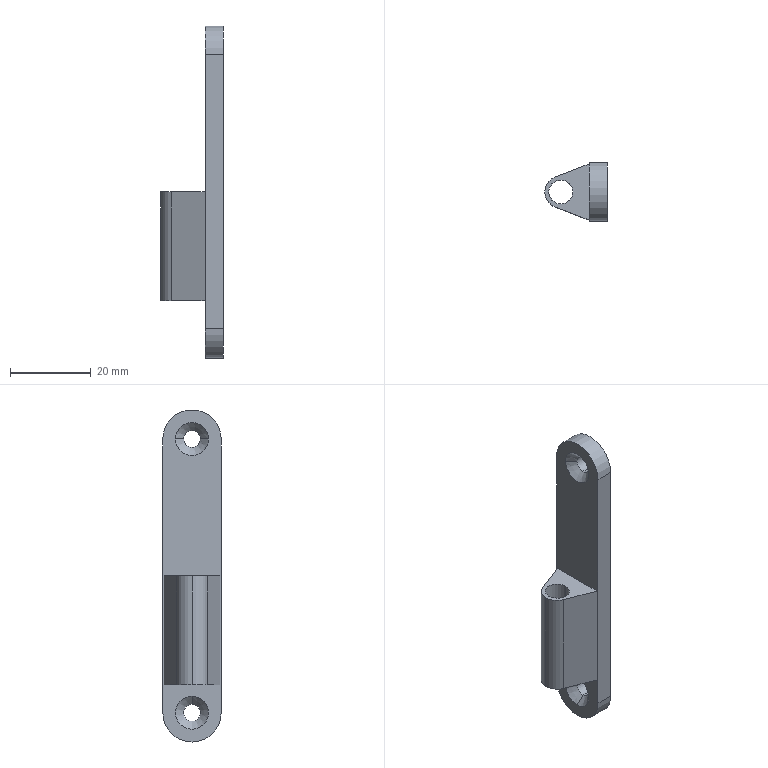Part | SolidWorks | features BaseBody 1 | 1 solid | 23 faces | box 15.5 x 14.5 x 82.5 mm | volume 7031 mm3 | cylinder 11 | plane 8 | cone 4 | commonest cylinder face diameters 4.2 x4 14.5 x3 6 x2 8 x2
STEP:
#1=CARTESIAN_POINT('',(11.5,0.,-36.1));
#2=VERTEX_POINT('',#1);
#3=CARTESIAN_POINT('',(11.5,0.,-31.9));
#4=VERTEX_POINT('',#3);
#5=CARTESIAN_POINT('',(11.5,0.,-34.));
#6=DIRECTION('',(-1.,0.,0.));
#7=DIRECTION('',(0.,0.,1.));
#8=AXIS2_PLACEMENT_3D('',#5,#6,#7);
#9=CIRCLE('',#8,2.1);
#10=EDGE_CURVE('',#2,#4,#9,.T.);
#11=ORIENTED_EDGE('',*,*,#10,.F.);
#12=CARTESIAN_POINT('',(9.,0.,-36.1));
#13=VERTEX_POINT('',#12);
#14=CARTESIAN_POINT('',(11.5,0.,-36.1));
#15=DIRECTION('',(-1.,0.,0.));
#16=VECTOR('',#15,1000.);
#17=LINE('',#14,#16);
#18=EDGE_CURVE('',#2,#13,#17,.T.);
#19=ORIENTED_EDGE('',*,*,#18,.T.);
#20=CARTESIAN_POINT('',(9.,0.,-31.9));
#21=VERTEX_POINT('',#20);
#22=CARTESIAN_POINT('',(9.,0.,-34.));
#23=DIRECTION('',(1.,0.,0.));
#24=DIRECTION('',(0.,0.,1.));
#25=AXIS2_PLACEMENT_3D('',#22,#23,#24);
#26=CIRCLE('',#25,2.1);
#27=EDGE_CURVE('',#21,#13,#26,.T.);
#28=ORIENTED_EDGE('',*,*,#27,.F.);
#29=CARTESIAN_POINT('',(11.5,0.,-31.9));
#30=DIRECTION('',(-1.,0.,0.));
#31=VECTOR('',#30,1000.);
#32=LINE('',#29,#31);
#33=EDGE_CURVE('',#4,#21,#32,.T.);
#34=ORIENTED_EDGE('',*,*,#33,.F.);
#35=EDGE_LOOP('',(#11,#19,#28,#34));
#36=FACE_OUTER_BOUND('',#35,.T.);
#37=CARTESIAN_POINT('',(11.5,0.,-34.));
#38=DIRECTION('',(-1.,0.,0.));
#39=DIRECTION('',(0.,0.,1.));
#40=AXIS2_PLACEMENT_3D('',#37,#38,#39);
#41=CYLINDRICAL_SURFACE('',#40,2.1);
#42=ADVANCED_FACE('',(#36),#41,.F.);
#43=CARTESIAN_POINT('',(7.,-7.25,-34.));
#44=VERTEX_POINT('',#43);
#45=CARTESIAN_POINT('',(7.,0.,-41.25));
#46=VERTEX_POINT('',#45);
#47=CARTESIAN_POINT('',(7.,0.,-34.));
#48=DIRECTION('',(1.,0.,0.));
#49=DIRECTION('',(0.,0.,-1.));
#50=AXIS2_PLACEMENT_3D('',#47,#48,#49);
#51=CIRCLE('',#50,7.25);
#52=EDGE_CURVE('',#44,#46,#51,.T.);
#53=ORIENTED_EDGE('',*,*,#52,.T.);
#54=CARTESIAN_POINT('',(11.5,0.,-41.25));
#55=VERTEX_POINT('',#54);
#56=CARTESIAN_POINT('',(11.5,0.,-41.25));
#57=DIRECTION('',(1.,0.,0.));
#58=VECTOR('',#57,1000.);
#59=LINE('',#56,#58);
#60=EDGE_CURVE('',#46,#55,#59,.T.);
#61=ORIENTED_EDGE('',*,*,#60,.T.);
#62=CARTESIAN_POINT('',(11.5,-7.25,-34.));
#63=VERTEX_POINT('',#62);
#64=CARTESIAN_POINT('',(11.5,0.,-34.));
#65=DIRECTION('',(1.,0.,0.));
#66=DIRECTION('',(0.,0.,-1.));
#67=AXIS2_PLACEMENT_3D('',#64,#65,#66);
#68=CIRCLE('',#67,7.25);
#69=EDGE_CURVE('',#63,#55,#68,.T.);
#70=ORIENTED_EDGE('',*,*,#69,.F.);
#71=CARTESIAN_POINT('',(11.5,-7.25,-34.));
#72=DIRECTION('',(-1.,0.,0.));
#73=VECTOR('',#72,1000.);
#74=LINE('',#71,#73);
#75=EDGE_CURVE('',#63,#44,#74,.T.);
#76=ORIENTED_EDGE('',*,*,#75,.T.);
#77=EDGE_LOOP('',(#53,#61,#70,#76));
#78=FACE_OUTER_BOUND('',#77,.T.);
#79=CARTESIAN_POINT('',(11.5,0.,-34.));
#80=DIRECTION('',(1.,0.,0.));
#81=DIRECTION('',(0.,0.,-1.));
#82=AXIS2_PLACEMENT_3D('',#79,#80,#81);
#83=CYLINDRICAL_SURFACE('',#82,7.25);
#84=ADVANCED_FACE('',(#78),#83,.T.);
#85=CARTESIAN_POINT('',(11.5,0.,31.9));
#86=VERTEX_POINT('',#85);
#87=CARTESIAN_POINT('',(11.5,0.,36.1));
#88=VERTEX_POINT('',#87);
#89=CARTESIAN_POINT('',(11.5,0.,34.));
#90=DIRECTION('',(-1.,0.,0.));
#91=DIRECTION('',(0.,0.,1.));
#92=AXIS2_PLACEMENT_3D('',#89,#90,#91);
#93=CIRCLE('',#92,2.1);
#94=EDGE_CURVE('',#86,#88,#93,.T.);
#95=ORIENTED_EDGE('',*,*,#94,.F.);
#96=CARTESIAN_POINT('',(9.,0.,31.9));
#97=VERTEX_POINT('',#96);
#98=CARTESIAN_POINT('',(11.5,0.,31.9));
#99=DIRECTION('',(-1.,0.,0.));
#100=VECTOR('',#99,1000.);
#101=LINE('',#98,#100);
#102=EDGE_CURVE('',#86,#97,#101,.T.);
#103=ORIENTED_EDGE('',*,*,#102,.T.);
#104=CARTESIAN_POINT('',(9.,-2.1,34.));
#105=VERTEX_POINT('',#104);
#106=CARTESIAN_POINT('',(9.,0.,34.));
#107=DIRECTION('',(1.,0.,0.));
#108=DIRECTION('',(0.,0.,1.));
#109=AXIS2_PLACEMENT_3D('',#106,#107,#108);
#110=CIRCLE('',#109,2.1);
#111=EDGE_CURVE('',#105,#97,#110,.T.);
#112=ORIENTED_EDGE('',*,*,#111,.F.);
#113=CARTESIAN_POINT('',(9.,0.,36.1));
#114=VERTEX_POINT('',#113);
#115=CARTESIAN_POINT('',(9.,0.,34.));
#116=DIRECTION('',(1.,0.,0.));
#117=DIRECTION('',(0.,0.,1.));
#118=AXIS2_PLACEMENT_3D('',#115,#116,#117);
#119=CIRCLE('',#118,2.1);
#120=EDGE_CURVE('',#114,#105,#119,.T.);
#121=ORIENTED_EDGE('',*,*,#120,.F.);
#122=CARTESIAN_POINT('',(11.5,0.,36.1));
#123=DIRECTION('',(-1.,0.,0.));
#124=VECTOR('',#123,1000.);
#125=LINE('',#122,#124);
#126=EDGE_CURVE('',#88,#114,#125,.T.);
#127=ORIENTED_EDGE('',*,*,#126,.F.);
#128=EDGE_LOOP('',(#95,#103,#112,#121,#127));
#129=FACE_OUTER_BOUND('',#128,.T.);
#130=CARTESIAN_POINT('',(11.5,0.,34.));
#131=DIRECTION('',(-1.,0.,0.));
#132=DIRECTION('',(0.,0.,1.));
#133=AXIS2_PLACEMENT_3D('',#130,#131,#132);
#134=CYLINDRICAL_SURFACE('',#133,2.1);
#135=ADVANCED_FACE('',(#129),#134,.F.);
#136=ORIENTED_EDGE('',*,*,#27,.T.);
#137=CARTESIAN_POINT('',(7.,0.,-38.1));
#138=VERTEX_POINT('',#137);
#139=CARTESIAN_POINT('',(7.,0.,-38.1));
#140=DIRECTION('',(-0.7071,0.,-0.7071));
#141=VECTOR('',#140,1000.);
#142=LINE('',#139,#141);
#143=EDGE_CURVE('',#13,#138,#142,.T.);
#144=ORIENTED_EDGE('',*,*,#143,.T.);
#145=CARTESIAN_POINT('',(7.,0.,-29.9));
#146=VERTEX_POINT('',#145);
#147=CARTESIAN_POINT('',(7.,0.,-34.));
#148=DIRECTION('',(1.,0.,0.));
#149=DIRECTION('',(0.,0.,1.));
#150=AXIS2_PLACEMENT_3D('',#147,#148,#149);
#151=CIRCLE('',#150,4.1);
#152=EDGE_CURVE('',#146,#138,#151,.T.);
#153=ORIENTED_EDGE('',*,*,#152,.F.);
#154=CARTESIAN_POINT('',(7.,0.,-29.9));
#155=DIRECTION('',(-0.7071,0.,0.7071));
#156=VECTOR('',#155,1000.);
#157=LINE('',#154,#156);
#158=EDGE_CURVE('',#21,#146,#157,.T.);
#159=ORIENTED_EDGE('',*,*,#158,.F.);
#160=EDGE_LOOP('',(#136,#144,#153,#159));
#161=FACE_OUTER_BOUND('',#160,.T.);
#162=CARTESIAN_POINT('',(7.,0.,-34.));
#163=DIRECTION('',(-1.,0.,0.));
#164=DIRECTION('',(0.,0.,1.));
#165=AXIS2_PLACEMENT_3D('',#162,#163,#164);
#166=CONICAL_SURFACE('',#165,4.1,0.7854);
#167=ADVANCED_FACE('',(#161),#166,.F.);
#168=ORIENTED_EDGE('',*,*,#111,.T.);
#169=CARTESIAN_POINT('',(9.,2.1,34.));
#170=VERTEX_POINT('',#169);
#171=CARTESIAN_POINT('',(9.,0.,34.));
#172=DIRECTION('',(1.,0.,0.));
#173=DIRECTION('',(0.,0.,1.));
#174=AXIS2_PLACEMENT_3D('',#171,#172,#173);
#175=CIRCLE('',#174,2.1);
#176=EDGE_CURVE('',#97,#170,#175,.T.);
#177=ORIENTED_EDGE('',*,*,#176,.T.);
#178=CARTESIAN_POINT('',(7.,4.1,34.));
#179=VERTEX_POINT('',#178);
#180=CARTESIAN_POINT('',(7.,4.1,34.));
#181=DIRECTION('',(-0.7071,0.7071,0.));
#182=VECTOR('',#181,1000.);
#183=LINE('',#180,#182);
#184=EDGE_CURVE('',#170,#179,#183,.T.);
#185=ORIENTED_EDGE('',*,*,#184,.T.);
#186=CARTESIAN_POINT('',(7.,-4.1,34.));
#187=VERTEX_POINT('',#186);
#188=CARTESIAN_POINT('',(7.,0.,34.));
#189=DIRECTION('',(-1.,0.,0.));
#190=DIRECTION('',(0.,-1.,0.));
#191=AXIS2_PLACEMENT_3D('',#188,#189,#190);
#192=CIRCLE('',#191,4.1);
#193=EDGE_CURVE('',#179,#187,#192,.T.);
#194=ORIENTED_EDGE('',*,*,#193,.T.);
#195=CARTESIAN_POINT('',(7.,-4.1,34.));
#196=DIRECTION('',(-0.7071,-0.7071,0.));
#197=VECTOR('',#196,1000.);
#198=LINE('',#195,#197);
#199=EDGE_CURVE('',#105,#187,#198,.T.);
#200=ORIENTED_EDGE('',*,*,#199,.F.);
#201=EDGE_LOOP('',(#168,#177,#185,#194,#200));
#202=FACE_OUTER_BOUND('',#201,.T.);
#203=CARTESIAN_POINT('',(7.,0.,34.));
#204=DIRECTION('',(-1.,0.,0.));
#205=DIRECTION('',(0.,-1.,0.));
#206=AXIS2_PLACEMENT_3D('',#203,#204,#205);
#207=CONICAL_SURFACE('',#206,4.1,0.7854);
#208=ADVANCED_FACE('',(#202),#207,.F.);
#209=CARTESIAN_POINT('',(-4.,0.,0.));
#210=VERTEX_POINT('',#209);
#211=CARTESIAN_POINT('',(-1.425,-3.738,0.));
#212=VERTEX_POINT('',#211);
#213=CARTESIAN_POINT('',(0.,0.,0.));
#214=DIRECTION('',(0.,0.,1.));
#215=DIRECTION('',(-1.,0.,0.));
#216=AXIS2_PLACEMENT_3D('',#213,#214,#215);
#217=CIRCLE('',#216,4.);
#218=EDGE_CURVE('',#210,#212,#217,.T.);
#219=ORIENTED_EDGE('',*,*,#218,.F.);
#220=CARTESIAN_POINT('',(-4.,0.,-27.));
#221=VERTEX_POINT('',#220);
#222=CARTESIAN_POINT('',(-4.,0.,-27.));
#223=DIRECTION('',(0.,0.,-1.));
#224=VECTOR('',#223,1000.);
#225=LINE('',#222,#224);
#226=EDGE_CURVE('',#210,#221,#225,.T.);
#227=ORIENTED_EDGE('',*,*,#226,.T.);
#228=CARTESIAN_POINT('',(-1.425,-3.738,-27.));
#229=VERTEX_POINT('',#228);
#230=CARTESIAN_POINT('',(0.,0.,-27.));
#231=DIRECTION('',(0.,0.,1.));
#232=DIRECTION('',(-1.,0.,0.));
#233=AXIS2_PLACEMENT_3D('',#230,#231,#232);
#234=CIRCLE('',#233,4.);
#235=EDGE_CURVE('',#221,#229,#234,.T.);
#236=ORIENTED_EDGE('',*,*,#235,.T.);
#237=CARTESIAN_POINT('',(-1.425,-3.738,-27.));
#238=DIRECTION('',(0.,0.,-1.));
#239=VECTOR('',#238,1000.);
#240=LINE('',#237,#239);
#241=EDGE_CURVE('',#212,#229,#240,.T.);
#242=ORIENTED_EDGE('',*,*,#241,.F.);
#243=EDGE_LOOP('',(#219,#227,#236,#242));
#244=FACE_OUTER_BOUND('',#243,.T.);
#245=CARTESIAN_POINT('',(0.,0.,-27.));
#246=DIRECTION('',(0.,0.,-1.));
#247=DIRECTION('',(-1.,0.,0.));
#248=AXIS2_PLACEMENT_3D('',#245,#246,#247);
#249=CYLINDRICAL_SURFACE('',#248,4.);
#250=ADVANCED_FACE('',(#244),#249,.T.);
#251=CARTESIAN_POINT('',(3.,0.,0.));
#252=VERTEX_POINT('',#251);
#253=CARTESIAN_POINT('',(-3.,0.,0.));
#254=VERTEX_POINT('',#253);
#255=CARTESIAN_POINT('',(0.,0.,0.));
#256=DIRECTION('',(0.,0.,-1.));
#257=DIRECTION('',(-1.,0.,0.));
#258=AXIS2_PLACEMENT_3D('',#255,#256,#257);
#259=CIRCLE('',#258,3.);
#260=EDGE_CURVE('',#252,#254,#259,.T.);
#261=ORIENTED_EDGE('',*,*,#260,.F.);
#262=CARTESIAN_POINT('',(3.,0.,-27.));
#263=VERTEX_POINT('',#262);
#264=CARTESIAN_POINT('',(3.,0.,-27.));
#265=DIRECTION('',(0.,0.,-1.));
#266=VECTOR('',#265,1000.);
#267=LINE('',#264,#266);
#268=EDGE_CURVE('',#252,#263,#267,.T.);
#269=ORIENTED_EDGE('',*,*,#268,.T.);
#270=CARTESIAN_POINT('',(-3.,0.,-27.));
#271=VERTEX_POINT('',#270);
#272=CARTESIAN_POINT('',(0.,0.,-27.));
#273=DIRECTION('',(0.,0.,-1.));
#274=DIRECTION('',(-1.,0.,0.));
#275=AXIS2_PLACEMENT_3D('',#272,#273,#274);
#276=CIRCLE('',#275,3.);
#277=EDGE_CURVE('',#263,#271,#276,.T.);
#278=ORIENTED_EDGE('',*,*,#277,.T.);
#279=CARTESIAN_POINT('',(-3.,0.,-27.));
#280=DIRECTION('',(0.,0.,-1.));
#281=VECTOR('',#280,1000.);
#282=LINE('',#279,#281);
#283=EDGE_CURVE('',#254,#271,#282,.T.);
#284=ORIENTED_EDGE('',*,*,#283,.F.);
#285=EDGE_LOOP('',(#261,#269,#278,#284));
#286=FACE_OUTER_BOUND('',#285,.T.);
#287=CARTESIAN_POINT('',(0.,0.,-27.));
#288=DIRECTION('',(0.,0.,-1.));
#289=DIRECTION('',(-1.,0.,0.));
#290=AXIS2_PLACEMENT_3D('',#287,#288,#289);
#291=CYLINDRICAL_SURFACE('',#290,3.);
#292=ADVANCED_FACE('',(#286),#291,.F.);
#293=CARTESIAN_POINT('',(11.5,0.,-34.));
#294=DIRECTION('',(-1.,0.,0.));
#295=DIRECTION('',(0.,0.,1.));
#296=AXIS2_PLACEMENT_3D('',#293,#294,#295);
#297=CIRCLE('',#296,2.1);
#298=EDGE_CURVE('',#4,#2,#297,.T.);
#299=ORIENTED_EDGE('',*,*,#298,.T.);
#300=ORIENTED_EDGE('',*,*,#10,.T.);
#301=EDGE_LOOP('',(#299,#300));
#302=FACE_BOUND('',#301,.T.);
#303=CARTESIAN_POINT('',(11.5,-7.25,34.));
#304=VERTEX_POINT('',#303);
#305=CARTESIAN_POINT('',(11.5,-7.25,34.));
#306=DIRECTION('',(0.,0.,-1.));
#307=VECTOR('',#306,1000.);
#308=LINE('',#305,#307);
#309=EDGE_CURVE('',#304,#63,#308,.T.);
#310=ORIENTED_EDGE('',*,*,#309,.T.);
#311=ORIENTED_EDGE('',*,*,#69,.T.);
#312=CARTESIAN_POINT('',(11.5,7.25,-34.));
#313=VERTEX_POINT('',#312);
#314=CARTESIAN_POINT('',(11.5,0.,-34.));
#315=DIRECTION('',(1.,0.,0.));
#316=DIRECTION('',(0.,0.,-1.));
#317=AXIS2_PLACEMENT_3D('',#314,#315,#316);
#318=CIRCLE('',#317,7.25);
#319=EDGE_CURVE('',#55,#313,#318,.T.);
#320=ORIENTED_EDGE('',*,*,#319,.T.);
#321=CARTESIAN_POINT('',(11.5,7.25,34.));
#322=VERTEX_POINT('',#321);
#323=CARTESIAN_POINT('',(11.5,7.25,34.));
#324=DIRECTION('',(0.,0.,1.));
#325=VECTOR('',#324,1000.);
#326=LINE('',#323,#325);
#327=EDGE_CURVE('',#313,#322,#326,.T.);
#328=ORIENTED_EDGE('',*,*,#327,.T.);
#329=CARTESIAN_POINT('',(11.5,0.,34.));
#330=DIRECTION('',(1.,0.,0.));
#331=DIRECTION('',(0.,0.,-1.));
#332=AXIS2_PLACEMENT_3D('',#329,#330,#331);
#333=CIRCLE('',#332,7.25);
#334=EDGE_CURVE('',#322,#304,#333,.T.);
#335=ORIENTED_EDGE('',*,*,#334,.T.);
#336=EDGE_LOOP('',(#310,#311,#320,#328,#335));
#337=FACE_OUTER_BOUND('',#336,.T.);
#338=CARTESIAN_POINT('',(11.5,0.,34.));
#339=DIRECTION('',(-1.,0.,0.));
#340=DIRECTION('',(0.,0.,1.));
#341=AXIS2_PLACEMENT_3D('',#338,#339,#340);
#342=CIRCLE('',#341,2.1);
#343=EDGE_CURVE('',#88,#86,#342,.T.);
#344=ORIENTED_EDGE('',*,*,#343,.T.);
#345=ORIENTED_EDGE('',*,*,#94,.T.);
#346=EDGE_LOOP('',(#344,#345));
#347=FACE_BOUND('',#346,.T.);
#348=CARTESIAN_POINT('',(11.5,0.,34.));
#349=DIRECTION('',(1.,0.,0.));
#350=DIRECTION('',(0.,0.,-1.));
#351=AXIS2_PLACEMENT_3D('',#348,#349,#350);
#352=PLANE('',#351);
#353=ADVANCED_FACE('',(#302,#337,#347),#352,.T.);
#354=ORIENTED_EDGE('',*,*,#18,.F.);
#355=ORIENTED_EDGE('',*,*,#298,.F.);
#356=ORIENTED_EDGE('',*,*,#33,.T.);
#357=CARTESIAN_POINT('',(9.,0.,-34.));
#358=DIRECTION('',(1.,0.,0.));
#359=DIRECTION('',(0.,0.,1.));
#360=AXIS2_PLACEMENT_3D('',#357,#358,#359);
#361=CIRCLE('',#360,2.1);
#362=EDGE_CURVE('',#13,#21,#361,.T.);
#363=ORIENTED_EDGE('',*,*,#362,.F.);
#364=EDGE_LOOP('',(#354,#355,#356,#363));
#365=FACE_OUTER_BOUND('',#364,.T.);
#366=CARTESIAN_POINT('',(11.5,0.,-34.));
#367=DIRECTION('',(-1.,0.,0.));
#368=DIRECTION('',(0.,0.,1.));
#369=AXIS2_PLACEMENT_3D('',#366,#367,#368);
#370=CYLINDRICAL_SURFACE('',#369,2.1);
#371=ADVANCED_FACE('',(#365),#370,.F.);
#372=ORIENTED_EDGE('',*,*,#60,.F.);
#373=CARTESIAN_POINT('',(7.,7.25,-34.));
#374=VERTEX_POINT('',#373);
#375=CARTESIAN_POINT('',(7.,0.,-34.));
#376=DIRECTION('',(1.,0.,0.));
#377=DIRECTION('',(0.,0.,-1.));
#378=AXIS2_PLACEMENT_3D('',#375,#376,#377);
#379=CIRCLE('',#378,7.25);
#380=EDGE_CURVE('',#46,#374,#379,.T.);
#381=ORIENTED_EDGE('',*,*,#380,.T.);
#382=CARTESIAN_POINT('',(11.5,7.25,-34.));
#383=DIRECTION('',(1.,0.,0.));
#384=VECTOR('',#383,1000.);
#385=LINE('',#382,#384);
#386=EDGE_CURVE('',#374,#313,#385,.T.);
#387=ORIENTED_EDGE('',*,*,#386,.T.);
#388=ORIENTED_EDGE('',*,*,#319,.F.);
#389=EDGE_LOOP('',(#372,#381,#387,#388));
#390=FACE_OUTER_BOUND('',#389,.T.);
#391=CARTESIAN_POINT('',(11.5,0.,-34.));
#392=DIRECTION('',(1.,0.,0.));
#393=DIRECTION('',(0.,0.,-1.));
#394=AXIS2_PLACEMENT_3D('',#391,#392,#393);
#395=CYLINDRICAL_SURFACE('',#394,7.25);
#396=ADVANCED_FACE('',(#390),#395,.T.);
#397=ORIENTED_EDGE('',*,*,#75,.F.);
#398=ORIENTED_EDGE('',*,*,#309,.F.);
#399=CARTESIAN_POINT('',(7.,-7.25,34.));
#400=VERTEX_POINT('',#399);
#401=CARTESIAN_POINT('',(11.5,-7.25,34.));
#402=DIRECTION('',(1.,0.,0.));
#403=VECTOR('',#402,1000.);
#404=LINE('',#401,#403);
#405=EDGE_CURVE('',#400,#304,#404,.T.);
#406=ORIENTED_EDGE('',*,*,#405,.F.);
#407=CARTESIAN_POINT('',(7.,-7.25,34.));
#408=DIRECTION('',(0.,0.,1.));
#409=VECTOR('',#408,1000.);
#410=LINE('',#407,#409);
#411=EDGE_CURVE('',#44,#400,#410,.T.);
#412=ORIENTED_EDGE('',*,*,#411,.F.);
#413=EDGE_LOOP('',(#397,#398,#406,#412));
#414=FACE_OUTER_BOUND('',#413,.T.);
#415=CARTESIAN_POINT('',(11.5,-7.25,34.));
#416=DIRECTION('',(0.,1.,0.));
#417=DIRECTION('',(0.,0.,1.));
#418=AXIS2_PLACEMENT_3D('',#415,#416,#417);
#419=PLANE('',#418);
#420=ADVANCED_FACE('',(#414),#419,.F.);
#421=ORIENTED_EDGE('',*,*,#334,.F.);
#422=CARTESIAN_POINT('',(7.,7.25,34.));
#423=VERTEX_POINT('',#422);
#424=CARTESIAN_POINT('',(11.5,7.25,34.));
#425=DIRECTION('',(-1.,0.,0.));
#426=VECTOR('',#425,1000.);
#427=LINE('',#424,#426);
#428=EDGE_CURVE('',#322,#423,#427,.T.);
#429=ORIENTED_EDGE('',*,*,#428,.T.);
#430=CARTESIAN_POINT('',(7.,0.,34.));
#431=DIRECTION('',(1.,0.,0.));
#432=DIRECTION('',(0.,0.,-1.));
#433=AXIS2_PLACEMENT_3D('',#430,#431,#432);
#434=CIRCLE('',#433,7.25);
#435=EDGE_CURVE('',#423,#400,#434,.T.);
#436=ORIENTED_EDGE('',*,*,#435,.T.);
#437=ORIENTED_EDGE('',*,*,#405,.T.);
#438=EDGE_LOOP('',(#421,#429,#436,#437));
#439=FACE_OUTER_BOUND('',#438,.T.);
#440=CARTESIAN_POINT('',(11.5,0.,34.));
#441=DIRECTION('',(1.,0.,0.));
#442=DIRECTION('',(0.,0.,-1.));
#443=AXIS2_PLACEMENT_3D('',#440,#441,#442);
#444=CYLINDRICAL_SURFACE('',#443,7.25);
#445=ADVANCED_FACE('',(#439),#444,.T.);
#446=ORIENTED_EDGE('',*,*,#428,.F.);
#447=ORIENTED_EDGE('',*,*,#327,.F.);
#448=ORIENTED_EDGE('',*,*,#386,.F.);
#449=CARTESIAN_POINT('',(7.,7.25,-34.));
#450=DIRECTION('',(0.,0.,-1.));
#451=VECTOR('',#450,1000.);
#452=LINE('',#449,#451);
#453=EDGE_CURVE('',#423,#374,#452,.T.);
#454=ORIENTED_EDGE('',*,*,#453,.F.);
#455=EDGE_LOOP('',(#446,#447,#448,#454));
#456=FACE_OUTER_BOUND('',#455,.T.);
#457=CARTESIAN_POINT('',(11.5,7.25,-34.));
#458=DIRECTION('',(0.,-1.,0.));
#459=DIRECTION('',(0.,0.,-1.));
#460=AXIS2_PLACEMENT_3D('',#457,#458,#459);
#461=PLANE('',#460);
#462=ADVANCED_FACE('',(#456),#461,.F.);
#463=ORIENTED_EDGE('',*,*,#102,.F.);
#464=ORIENTED_EDGE('',*,*,#343,.F.);
#465=ORIENTED_EDGE('',*,*,#126,.T.);
#466=CARTESIAN_POINT('',(9.,0.,34.));
#467=DIRECTION('',(1.,0.,0.));
#468=DIRECTION('',(0.,0.,1.));
#469=AXIS2_PLACEMENT_3D('',#466,#467,#468);
#470=CIRCLE('',#469,2.1);
#471=EDGE_CURVE('',#170,#114,#470,.T.);
#472=ORIENTED_EDGE('',*,*,#471,.F.);
#473=ORIENTED_EDGE('',*,*,#176,.F.);
#474=EDGE_LOOP('',(#463,#464,#465,#472,#473));
#475=FACE_OUTER_BOUND('',#474,.T.);
#476=CARTESIAN_POINT('',(11.5,0.,34.));
#477=DIRECTION('',(-1.,0.,0.));
#478=DIRECTION('',(0.,0.,1.));
#479=AXIS2_PLACEMENT_3D('',#476,#477,#478);
#480=CYLINDRICAL_SURFACE('',#479,2.1);
#481=ADVANCED_FACE('',(#475),#480,.F.);
#482=ORIENTED_EDGE('',*,*,#143,.F.);
#483=ORIENTED_EDGE('',*,*,#362,.T.);
#484=ORIENTED_EDGE('',*,*,#158,.T.);
#485=CARTESIAN_POINT('',(7.,0.,-34.));
#486=DIRECTION('',(1.,0.,0.));
#487=DIRECTION('',(0.,0.,1.));
#488=AXIS2_PLACEMENT_3D('',#485,#486,#487);
#489=CIRCLE('',#488,4.1);
#490=EDGE_CURVE('',#138,#146,#489,.T.);
#491=ORIENTED_EDGE('',*,*,#490,.F.);
#492=EDGE_LOOP('',(#482,#483,#484,#491));
#493=FACE_OUTER_BOUND('',#492,.T.);
#494=CARTESIAN_POINT('',(7.,0.,-34.));
#495=DIRECTION('',(-1.,0.,0.));
#496=DIRECTION('',(0.,0.,1.));
#497=AXIS2_PLACEMENT_3D('',#494,#495,#496);
#498=CONICAL_SURFACE('',#497,4.1,0.7854);
#499=ADVANCED_FACE('',(#493),#498,.F.);
#500=ORIENTED_EDGE('',*,*,#152,.T.);
#501=ORIENTED_EDGE('',*,*,#490,.T.);
#502=EDGE_LOOP('',(#500,#501));
#503=FACE_BOUND('',#502,.T.);
#504=CARTESIAN_POINT('',(7.,6.95,-27.));
#505=VERTEX_POINT('',#504);
#506=CARTESIAN_POINT('',(7.,-6.95,-27.));
#507=VERTEX_POINT('',#506);
#508=CARTESIAN_POINT('',(7.,0.,-27.));
#509=DIRECTION('',(0.,-1.,0.));
#510=VECTOR('',#509,1000.);
#511=LINE('',#508,#510);
#512=EDGE_CURVE('',#505,#507,#511,.T.);
#513=ORIENTED_EDGE('',*,*,#512,.F.);
#514=CARTESIAN_POINT('',(7.,6.95,0.));
#515=VERTEX_POINT('',#514);
#516=CARTESIAN_POINT('',(7.,6.95,34.));
#517=DIRECTION('',(0.,0.,-1.));
#518=VECTOR('',#517,1000.);
#519=LINE('',#516,#518);
#520=EDGE_CURVE('',#515,#505,#519,.T.);
#521=ORIENTED_EDGE('',*,*,#520,.F.);
#522=CARTESIAN_POINT('',(7.,-6.95,0.));
#523=VERTEX_POINT('',#522);
#524=CARTESIAN_POINT('',(7.,0.,0.));
#525=DIRECTION('',(0.,1.,0.));
#526=VECTOR('',#525,1000.);
#527=LINE('',#524,#526);
#528=EDGE_CURVE('',#523,#515,#527,.T.);
#529=ORIENTED_EDGE('',*,*,#528,.F.);
#530=CARTESIAN_POINT('',(7.,-6.95,34.));
#531=DIRECTION('',(0.,0.,1.));
#532=VECTOR('',#531,1000.);
#533=LINE('',#530,#532);
#534=EDGE_CURVE('',#507,#523,#533,.T.);
#535=ORIENTED_EDGE('',*,*,#534,.F.);
#536=EDGE_LOOP('',(#513,#521,#529,#535));
#537=FACE_BOUND('',#536,.T.);
#538=ORIENTED_EDGE('',*,*,#52,.F.);
#539=ORIENTED_EDGE('',*,*,#411,.T.);
#540=ORIENTED_EDGE('',*,*,#435,.F.);
#541=ORIENTED_EDGE('',*,*,#453,.T.);
#542=ORIENTED_EDGE('',*,*,#380,.F.);
#543=EDGE_LOOP('',(#538,#539,#540,#541,#542));
#544=FACE_OUTER_BOUND('',#543,.T.);
#545=CARTESIAN_POINT('',(7.,0.,34.));
#546=DIRECTION('',(-1.,0.,0.));
#547=DIRECTION('',(0.,-1.,0.));
#548=AXIS2_PLACEMENT_3D('',#545,#546,#547);
#549=CIRCLE('',#548,4.1);
#550=EDGE_CURVE('',#187,#179,#549,.T.);
#551=ORIENTED_EDGE('',*,*,#550,.F.);
#552=ORIENTED_EDGE('',*,*,#193,.F.);
#553=EDGE_LOOP('',(#551,#552));
#554=FACE_BOUND('',#553,.T.);
#555=CARTESIAN_POINT('',(7.,0.,34.));
#556=DIRECTION('',(1.,0.,0.));
#557=DIRECTION('',(0.,0.,-1.));
#558=AXIS2_PLACEMENT_3D('',#555,#556,#557);
#559=PLANE('',#558);
#560=ADVANCED_FACE('',(#503,#537,#544,#554),#559,.F.);
#561=ORIENTED_EDGE('',*,*,#184,.F.);
#562=ORIENTED_EDGE('',*,*,#471,.T.);
#563=ORIENTED_EDGE('',*,*,#120,.T.);
#564=ORIENTED_EDGE('',*,*,#199,.T.);
#565=ORIENTED_EDGE('',*,*,#550,.T.);
#566=EDGE_LOOP('',(#561,#562,#563,#564,#565));
#567=FACE_OUTER_BOUND('',#566,.T.);
#568=CARTESIAN_POINT('',(7.,0.,34.));
#569=DIRECTION('',(-1.,0.,0.));
#570=DIRECTION('',(0.,-1.,0.));
#571=AXIS2_PLACEMENT_3D('',#568,#569,#570);
#572=CONICAL_SURFACE('',#571,4.1,0.7854);
#573=ADVANCED_FACE('',(#567),#572,.F.);
#574=CARTESIAN_POINT('',(-1.425,-3.738,-27.));
#575=DIRECTION('',(0.9344,-0.3563,0.));
#576=VECTOR('',#575,1000.);
#577=LINE('',#574,#576);
#578=EDGE_CURVE('',#229,#507,#577,.T.);
#579=ORIENTED_EDGE('',*,*,#578,.T.);
#580=ORIENTED_EDGE('',*,*,#534,.T.);
#581=CARTESIAN_POINT('',(-1.425,-3.738,0.));
#582=DIRECTION('',(-0.9344,0.3563,0.));
#583=VECTOR('',#582,1000.);
#584=LINE('',#581,#583);
#585=EDGE_CURVE('',#523,#212,#584,.T.);
#586=ORIENTED_EDGE('',*,*,#585,.T.);
#587=ORIENTED_EDGE('',*,*,#241,.T.);
#588=EDGE_LOOP('',(#579,#580,#586,#587));
#589=FACE_OUTER_BOUND('',#588,.T.);
#590=CARTESIAN_POINT('',(-1.425,-3.738,-27.));
#591=DIRECTION('',(-0.3563,-0.9344,0.));
#592=DIRECTION('',(0.9344,-0.3563,0.));
#593=AXIS2_PLACEMENT_3D('',#590,#591,#592);
#594=PLANE('',#593);
#595=ADVANCED_FACE('',(#589),#594,.T.);
#596=ORIENTED_EDGE('',*,*,#512,.T.);
#597=ORIENTED_EDGE('',*,*,#578,.F.);
#598=ORIENTED_EDGE('',*,*,#235,.F.);
#599=CARTESIAN_POINT('',(-1.425,3.738,-27.));
#600=VERTEX_POINT('',#599);
#601=CARTESIAN_POINT('',(0.,0.,-27.));
#602=DIRECTION('',(0.,0.,1.));
#603=DIRECTION('',(-1.,0.,0.));
#604=AXIS2_PLACEMENT_3D('',#601,#602,#603);
#605=CIRCLE('',#604,4.);
#606=EDGE_CURVE('',#600,#221,#605,.T.);
#607=ORIENTED_EDGE('',*,*,#606,.F.);
#608=CARTESIAN_POINT('',(7.,6.95,-27.));
#609=DIRECTION('',(-0.9344,-0.3563,0.));
#610=VECTOR('',#609,1000.);
#611=LINE('',#608,#610);
#612=EDGE_CURVE('',#505,#600,#611,.T.);
#613=ORIENTED_EDGE('',*,*,#612,.F.);
#614=EDGE_LOOP('',(#596,#597,#598,#607,#613));
#615=FACE_OUTER_BOUND('',#614,.T.);
#616=CARTESIAN_POINT('',(0.,0.,-27.));
#617=DIRECTION('',(0.,0.,-1.));
#618=DIRECTION('',(-1.,0.,0.));
#619=AXIS2_PLACEMENT_3D('',#616,#617,#618);
#620=CIRCLE('',#619,3.);
#621=EDGE_CURVE('',#271,#263,#620,.T.);
#622=ORIENTED_EDGE('',*,*,#621,.F.);
#623=ORIENTED_EDGE('',*,*,#277,.F.);
#624=EDGE_LOOP('',(#622,#623));
#625=FACE_BOUND('',#624,.T.);
#626=CARTESIAN_POINT('',(0.,0.,-27.));
#627=DIRECTION('',(0.,0.,1.));
#628=DIRECTION('',(1.,0.,0.));
#629=AXIS2_PLACEMENT_3D('',#626,#627,#628);
#630=PLANE('',#629);
#631=ADVANCED_FACE('',(#615,#625),#630,.F.);
#632=ORIENTED_EDGE('',*,*,#612,.T.);
#633=CARTESIAN_POINT('',(-1.425,3.738,0.));
#634=VERTEX_POINT('',#633);
#635=CARTESIAN_POINT('',(-1.425,3.738,-27.));
#636=DIRECTION('',(0.,0.,1.));
#637=VECTOR('',#636,1000.);
#638=LINE('',#635,#637);
#639=EDGE_CURVE('',#600,#634,#638,.T.);
#640=ORIENTED_EDGE('',*,*,#639,.T.);
#641=CARTESIAN_POINT('',(7.,6.95,0.));
#642=DIRECTION('',(0.9344,0.3563,0.));
#643=VECTOR('',#642,1000.);
#644=LINE('',#641,#643);
#645=EDGE_CURVE('',#634,#515,#644,.T.);
#646=ORIENTED_EDGE('',*,*,#645,.T.);
#647=ORIENTED_EDGE('',*,*,#520,.T.);
#648=EDGE_LOOP('',(#632,#640,#646,#647));
#649=FACE_OUTER_BOUND('',#648,.T.);
#650=CARTESIAN_POINT('',(7.,6.95,-27.));
#651=DIRECTION('',(-0.3563,0.9344,0.));
#652=DIRECTION('',(-0.9344,-0.3563,0.));
#653=AXIS2_PLACEMENT_3D('',#650,#651,#652);
#654=PLANE('',#653);
#655=ADVANCED_FACE('',(#649),#654,.T.);
#656=ORIENTED_EDGE('',*,*,#585,.F.);
#657=ORIENTED_EDGE('',*,*,#528,.T.);
#658=ORIENTED_EDGE('',*,*,#645,.F.);
#659=CARTESIAN_POINT('',(0.,0.,0.));
#660=DIRECTION('',(0.,0.,1.));
#661=DIRECTION('',(-1.,0.,0.));
#662=AXIS2_PLACEMENT_3D('',#659,#660,#661);
#663=CIRCLE('',#662,4.);
#664=EDGE_CURVE('',#634,#210,#663,.T.);
#665=ORIENTED_EDGE('',*,*,#664,.T.);
#666=ORIENTED_EDGE('',*,*,#218,.T.);
#667=EDGE_LOOP('',(#656,#657,#658,#665,#666));
#668=FACE_OUTER_BOUND('',#667,.T.);
#669=CARTESIAN_POINT('',(0.,0.,0.));
#670=DIRECTION('',(0.,0.,-1.));
#671=DIRECTION('',(-1.,0.,0.));
#672=AXIS2_PLACEMENT_3D('',#669,#670,#671);
#673=CIRCLE('',#672,3.);
#674=EDGE_CURVE('',#254,#252,#673,.T.);
#675=ORIENTED_EDGE('',*,*,#674,.T.);
#676=ORIENTED_EDGE('',*,*,#260,.T.);
#677=EDGE_LOOP('',(#675,#676));
#678=FACE_BOUND('',#677,.T.);
#679=CARTESIAN_POINT('',(0.,0.,0.));
#680=DIRECTION('',(0.,0.,1.));
#681=DIRECTION('',(1.,0.,0.));
#682=AXIS2_PLACEMENT_3D('',#679,#680,#681);
#683=PLANE('',#682);
#684=ADVANCED_FACE('',(#668,#678),#683,.T.);
#685=ORIENTED_EDGE('',*,*,#226,.F.);
#686=ORIENTED_EDGE('',*,*,#664,.F.);
#687=ORIENTED_EDGE('',*,*,#639,.F.);
#688=ORIENTED_EDGE('',*,*,#606,.T.);
#689=EDGE_LOOP('',(#685,#686,#687,#688));
#690=FACE_OUTER_BOUND('',#689,.T.);
#691=CARTESIAN_POINT('',(0.,0.,-27.));
#692=DIRECTION('',(0.,0.,-1.));
#693=DIRECTION('',(-1.,0.,0.));
#694=AXIS2_PLACEMENT_3D('',#691,#692,#693);
#695=CYLINDRICAL_SURFACE('',#694,4.);
#696=ADVANCED_FACE('',(#690),#695,.T.);
#697=ORIENTED_EDGE('',*,*,#268,.F.);
#698=ORIENTED_EDGE('',*,*,#674,.F.);
#699=ORIENTED_EDGE('',*,*,#283,.T.);
#700=ORIENTED_EDGE('',*,*,#621,.T.);
#701=EDGE_LOOP('',(#697,#698,#699,#700));
#702=FACE_OUTER_BOUND('',#701,.T.);
#703=CARTESIAN_POINT('',(0.,0.,-27.));
#704=DIRECTION('',(0.,0.,-1.));
#705=DIRECTION('',(-1.,0.,0.));
#706=AXIS2_PLACEMENT_3D('',#703,#704,#705);
#707=CYLINDRICAL_SURFACE('',#706,3.);
#708=ADVANCED_FACE('',(#702),#707,.F.);
#709=CLOSED_SHELL('',(#42,#84,#135,#167,#208,#250,#292,#353,#371,#396,#420,#445,#462,#481,#499,#560,#573,#595,#631,#655,#684,#696,#708));
#710=MANIFOLD_SOLID_BREP('',#709);
#711=CARTESIAN_POINT('',(0.,0.,0.));
#712=DIRECTION('',(0.,0.,1.));
#713=DIRECTION('',(1.,0.,0.));
#714=AXIS2_PLACEMENT_3D('',#711,#712,#713);
#715=(LENGTH_UNIT()NAMED_UNIT(*)SI_UNIT(.MILLI.,.METRE.));
#716=UNCERTAINTY_MEASURE_WITH_UNIT(LENGTH_MEASURE(0.00001),#715,'','');
#717=(NAMED_UNIT(*)PLANE_ANGLE_UNIT()SI_UNIT($,.RADIAN.));
#718=(NAMED_UNIT(*)SI_UNIT($,.STERADIAN.)SOLID_ANGLE_UNIT());
#719=(GEOMETRIC_REPRESENTATION_CONTEXT(3)GLOBAL_UNCERTAINTY_ASSIGNED_CONTEXT((#716))GLOBAL_UNIT_ASSIGNED_CONTEXT((#715,#717,#718))REPRESENTATION_CONTEXT('',''));
#720=ADVANCED_BREP_SHAPE_REPRESENTATION('',(#710,#714),#719);